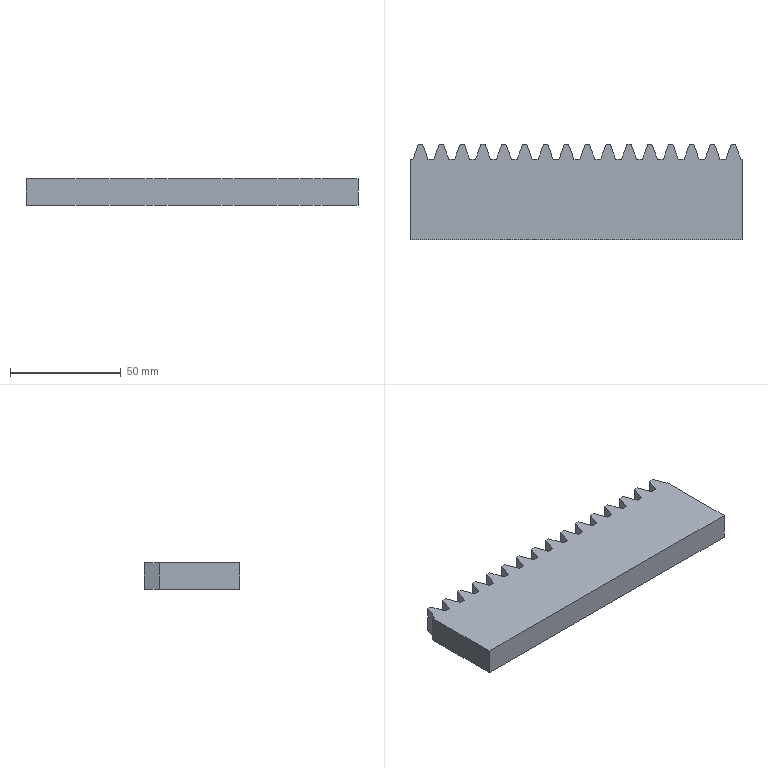Part | SolidWorks | features BaseBody 1 | 1 solid | 70 faces | box 150 x 43 x 12 mm | volume 70879 mm3 | plane 70